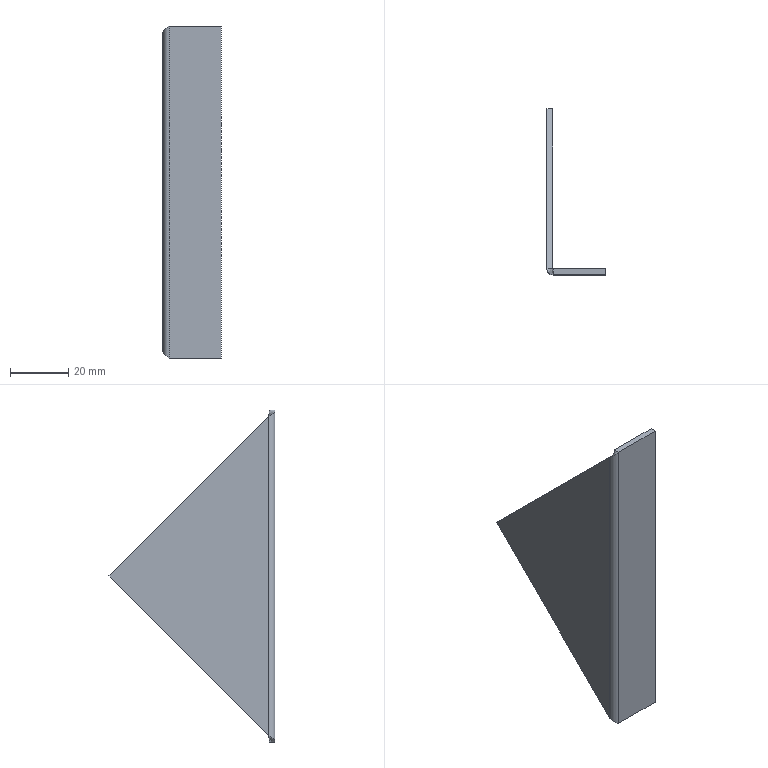Part | STEP file | Front Left Filler Piece | 1 solid | 13 faces | box 20 x 57.062 x 114.125 mm | volume 10515 mm3 | plane 9 | cylinder 2 | spline 2 | commonest cylinder face diameters 0.2 x1 4.2 x1
STEP:
#1=CARTESIAN_POINT('',(-2.,2.1,-54.962));
#2=VERTEX_POINT('',#1);
#3=CARTESIAN_POINT('',(-2.,2.1,54.962));
#4=VERTEX_POINT('',#3);
#5=CARTESIAN_POINT('',(-2.,2.1,0.));
#6=DIRECTION('',(0.,0.,1.));
#7=VECTOR('',#6,1000.);
#8=LINE('',#5,#7);
#9=EDGE_CURVE('',#2,#4,#8,.T.);
#10=ORIENTED_EDGE('',*,*,#9,.T.);
#11=CARTESIAN_POINT('',(-2.,57.062,0.));
#12=VERTEX_POINT('',#11);
#13=CARTESIAN_POINT('',(-2.,2.1,54.962));
#14=DIRECTION('',(0.,0.7071,-0.7071));
#15=VECTOR('',#14,1000.);
#16=LINE('',#13,#15);
#17=EDGE_CURVE('',#4,#12,#16,.T.);
#18=ORIENTED_EDGE('',*,*,#17,.T.);
#19=CARTESIAN_POINT('',(-2.,57.062,0.));
#20=DIRECTION('',(0.,-0.7071,-0.7071));
#21=VECTOR('',#20,1000.);
#22=LINE('',#19,#21);
#23=EDGE_CURVE('',#12,#2,#22,.T.);
#24=ORIENTED_EDGE('',*,*,#23,.T.);
#25=EDGE_LOOP('',(#10,#18,#24));
#26=FACE_OUTER_BOUND('',#25,.T.);
#27=CARTESIAN_POINT('',(-2.,0.,0.));
#28=DIRECTION('',(-1.,0.,0.));
#29=DIRECTION('',(0.,0.,1.));
#30=AXIS2_PLACEMENT_3D('',#27,#28,#29);
#31=PLANE('',#30);
#32=ADVANCED_FACE('',(#26),#31,.T.);
#33=CARTESIAN_POINT('',(0.,2.1,54.962));
#34=VERTEX_POINT('',#33);
#35=CARTESIAN_POINT('',(0.,57.062,0.));
#36=VERTEX_POINT('',#35);
#37=CARTESIAN_POINT('',(0.,57.062,0.));
#38=DIRECTION('',(0.,0.7071,-0.7071));
#39=VECTOR('',#38,1000.);
#40=LINE('',#37,#39);
#41=EDGE_CURVE('',#34,#36,#40,.T.);
#42=ORIENTED_EDGE('',*,*,#41,.T.);
#43=CARTESIAN_POINT('',(-2.,57.062,0.));
#44=DIRECTION('',(-1.,0.,0.));
#45=VECTOR('',#44,1000.);
#46=LINE('',#43,#45);
#47=EDGE_CURVE('',#36,#12,#46,.T.);
#48=ORIENTED_EDGE('',*,*,#47,.T.);
#49=ORIENTED_EDGE('',*,*,#17,.F.);
#50=CARTESIAN_POINT('',(-2.,2.1,54.962));
#51=DIRECTION('',(1.,0.,0.));
#52=VECTOR('',#51,1000.);
#53=LINE('',#50,#52);
#54=EDGE_CURVE('',#4,#34,#53,.T.);
#55=ORIENTED_EDGE('',*,*,#54,.T.);
#56=EDGE_LOOP('',(#42,#48,#49,#55));
#57=FACE_OUTER_BOUND('',#56,.T.);
#58=CARTESIAN_POINT('',(-2.,57.062,0.));
#59=DIRECTION('',(0.,0.7071,0.7071));
#60=DIRECTION('',(0.,-0.7071,0.7071));
#61=AXIS2_PLACEMENT_3D('',#58,#59,#60);
#62=PLANE('',#61);
#63=ADVANCED_FACE('',(#57),#62,.T.);
#64=CARTESIAN_POINT('',(0.1,0.,-57.062));
#65=VERTEX_POINT('',#64);
#66=CARTESIAN_POINT('',(0.1,0.,57.062));
#67=VERTEX_POINT('',#66);
#68=CARTESIAN_POINT('',(0.1,0.,-57.062));
#69=DIRECTION('',(0.,0.,1.));
#70=VECTOR('',#69,1000.);
#71=LINE('',#68,#70);
#72=EDGE_CURVE('',#65,#67,#71,.T.);
#73=ORIENTED_EDGE('',*,*,#72,.T.);
#74=CARTESIAN_POINT('',(0.1,0.,57.062));
#75=CARTESIAN_POINT('',(0.06419,0.,57.04));
#76=CARTESIAN_POINT('',(0.02837,0.0009165,57.017));
#77=CARTESIAN_POINT('',(-0.007394,0.002748,56.994));
#78=CARTESIAN_POINT('',(-0.04316,0.004579,56.971));
#79=CARTESIAN_POINT('',(-0.07888,0.007326,56.948));
#80=CARTESIAN_POINT('',(-0.1145,0.01098,56.926));
#81=CARTESIAN_POINT('',(-0.1501,0.01464,56.903));
#82=CARTESIAN_POINT('',(-0.1857,0.01921,56.88));
#83=CARTESIAN_POINT('',(-0.2211,0.02469,56.857));
#84=CARTESIAN_POINT('',(-0.2565,0.03016,56.834));
#85=CARTESIAN_POINT('',(-0.2917,0.03655,56.812));
#86=CARTESIAN_POINT('',(-0.3268,0.04382,56.789));
#87=CARTESIAN_POINT('',(-0.3618,0.0511,56.766));
#88=CARTESIAN_POINT('',(-0.3967,0.05928,56.743));
#89=CARTESIAN_POINT('',(-0.4314,0.06834,56.72));
#90=CARTESIAN_POINT('',(-0.466,0.0774,56.698));
#91=CARTESIAN_POINT('',(-0.5004,0.08735,56.675));
#92=CARTESIAN_POINT('',(-0.5346,0.09817,56.652));
#93=CARTESIAN_POINT('',(-0.5687,0.109,56.629));
#94=CARTESIAN_POINT('',(-0.6026,0.1207,56.606));
#95=CARTESIAN_POINT('',(-0.6361,0.1332,56.584));
#96=CARTESIAN_POINT('',(-0.6697,0.1458,56.561));
#97=CARTESIAN_POINT('',(-0.7029,0.1592,56.538));
#98=CARTESIAN_POINT('',(-0.7357,0.1735,56.515));
#99=CARTESIAN_POINT('',(-0.7686,0.1877,56.492));
#100=CARTESIAN_POINT('',(-0.8011,0.2028,56.47));
#101=CARTESIAN_POINT('',(-0.8332,0.2187,56.447));
#102=CARTESIAN_POINT('',(-0.8652,0.2346,56.424));
#103=CARTESIAN_POINT('',(-0.8969,0.2514,56.401));
#104=CARTESIAN_POINT('',(-0.9282,0.2689,56.378));
#105=CARTESIAN_POINT('',(-0.9594,0.2864,56.356));
#106=CARTESIAN_POINT('',(-0.9902,0.3048,56.333));
#107=CARTESIAN_POINT('',(-1.02,0.3239,56.31));
#108=CARTESIAN_POINT('',(-1.051,0.343,56.287));
#109=CARTESIAN_POINT('',(-1.081,0.3629,56.264));
#110=CARTESIAN_POINT('',(-1.11,0.3835,56.242));
#111=CARTESIAN_POINT('',(-1.139,0.4041,56.219));
#112=CARTESIAN_POINT('',(-1.168,0.4255,56.196));
#113=CARTESIAN_POINT('',(-1.196,0.4476,56.173));
#114=CARTESIAN_POINT('',(-1.224,0.4697,56.15));
#115=CARTESIAN_POINT('',(-1.252,0.4926,56.128));
#116=CARTESIAN_POINT('',(-1.279,0.5161,56.105));
#117=CARTESIAN_POINT('',(-1.306,0.5396,56.082));
#118=CARTESIAN_POINT('',(-1.332,0.5638,56.059));
#119=CARTESIAN_POINT('',(-1.358,0.5887,56.036));
#120=CARTESIAN_POINT('',(-1.384,0.6135,56.014));
#121=CARTESIAN_POINT('',(-1.409,0.639,55.991));
#122=CARTESIAN_POINT('',(-1.433,0.6652,55.968));
#123=CARTESIAN_POINT('',(-1.458,0.6913,55.945));
#124=CARTESIAN_POINT('',(-1.482,0.7181,55.922));
#125=CARTESIAN_POINT('',(-1.505,0.7455,55.9));
#126=CARTESIAN_POINT('',(-1.528,0.7729,55.877));
#127=CARTESIAN_POINT('',(-1.55,0.8008,55.854));
#128=CARTESIAN_POINT('',(-1.572,0.8293,55.831));
#129=CARTESIAN_POINT('',(-1.594,0.8578,55.808));
#130=CARTESIAN_POINT('',(-1.615,0.8869,55.786));
#131=CARTESIAN_POINT('',(-1.635,0.9165,55.763));
#132=CARTESIAN_POINT('',(-1.655,0.9461,55.74));
#133=CARTESIAN_POINT('',(-1.674,0.9762,55.717));
#134=CARTESIAN_POINT('',(-1.693,1.007,55.694));
#135=CARTESIAN_POINT('',(-1.712,1.037,55.672));
#136=CARTESIAN_POINT('',(-1.73,1.068,55.649));
#137=CARTESIAN_POINT('',(-1.747,1.1,55.626));
#138=CARTESIAN_POINT('',(-1.764,1.131,55.603));
#139=CARTESIAN_POINT('',(-1.78,1.163,55.58));
#140=CARTESIAN_POINT('',(-1.795,1.196,55.558));
#141=CARTESIAN_POINT('',(-1.811,1.228,55.535));
#142=CARTESIAN_POINT('',(-1.825,1.261,55.512));
#143=CARTESIAN_POINT('',(-1.839,1.294,55.489));
#144=CARTESIAN_POINT('',(-1.846,1.31,55.478));
#145=CARTESIAN_POINT('',(-1.853,1.327,55.466));
#146=CARTESIAN_POINT('',(-1.859,1.344,55.455));
#147=CARTESIAN_POINT('',(-1.872,1.377,55.432));
#148=CARTESIAN_POINT('',(-1.884,1.411,55.409));
#149=CARTESIAN_POINT('',(-1.895,1.445,55.387));
#150=CARTESIAN_POINT('',(-1.906,1.479,55.364));
#151=CARTESIAN_POINT('',(-1.917,1.513,55.341));
#152=CARTESIAN_POINT('',(-1.926,1.548,55.318));
#153=CARTESIAN_POINT('',(-1.935,1.582,55.295));
#154=CARTESIAN_POINT('',(-1.944,1.617,55.273));
#155=CARTESIAN_POINT('',(-1.952,1.652,55.25));
#156=CARTESIAN_POINT('',(-1.959,1.687,55.227));
#157=CARTESIAN_POINT('',(-1.966,1.722,55.204));
#158=CARTESIAN_POINT('',(-1.972,1.758,55.181));
#159=CARTESIAN_POINT('',(-1.978,1.793,55.159));
#160=CARTESIAN_POINT('',(-1.983,1.828,55.136));
#161=CARTESIAN_POINT('',(-1.987,1.864,55.113));
#162=CARTESIAN_POINT('',(-1.991,1.903,55.088));
#163=CARTESIAN_POINT('',(-1.994,1.942,55.063));
#164=CARTESIAN_POINT('',(-1.997,1.982,55.038));
#165=CARTESIAN_POINT('',(-1.999,2.021,55.013));
#166=CARTESIAN_POINT('',(-2.,2.061,54.988));
#167=CARTESIAN_POINT('',(-2.,2.1,54.962));
#168=B_SPLINE_CURVE_WITH_KNOTS('',3,(#74,#75,#76,#77,#78,#79,#80,#81,#82,#83,#84,#85,#86,#87,#88,#89,#90,#91,#92,#93,#94,#95,#96,#97,#98,#99,#100,#101,#102,#103,#104,#105,#106,#107,#108,#109,#110,#111,#112,#113,#114,#115,#116,#117,#118,#119,#120,#121,#122,#123,#124,#125,#126,#127,#128,#129,#130,#131,#132,#133,#134,#135,#136,#137,#138,#139,#140,#141,#142,#143,#144,#145,#146,#147,#148,#149,#150,#151,#152,#153,#154,#155,#156,#157,#158,#159,#160,#161,#162,#163,#164,#165,#166,#167),.UNSPECIFIED.,.F.,.F.,(4,3,3,3,3,3,3,3,3,3,3,3,3,3,3,3,3,3,3,3,3,3,3,3,3,3,3,3,3,3,3,4),(0.,0.0001274,0.0002547,0.0003821,0.0005094,0.0006368,0.0007641,0.0008915,0.001019,0.001146,0.001274,0.001401,0.001528,0.001656,0.001783,0.00191,0.002038,0.002165,0.002292,0.00242,0.002547,0.002674,0.002802,0.002929,0.002993,0.00312,0.003248,0.003375,0.003502,0.00363,0.00377,0.00391),.UNSPECIFIED.);
#169=EDGE_CURVE('',#67,#4,#168,.T.);
#170=ORIENTED_EDGE('',*,*,#169,.T.);
#171=ORIENTED_EDGE('',*,*,#9,.F.);
#172=CARTESIAN_POINT('',(-2.,2.1,-54.962));
#173=CARTESIAN_POINT('',(-2.,2.064,-54.985));
#174=CARTESIAN_POINT('',(-1.999,2.028,-55.008));
#175=CARTESIAN_POINT('',(-1.997,1.993,-55.031));
#176=CARTESIAN_POINT('',(-1.995,1.957,-55.054));
#177=CARTESIAN_POINT('',(-1.993,1.921,-55.076));
#178=CARTESIAN_POINT('',(-1.989,1.885,-55.099));
#179=CARTESIAN_POINT('',(-1.985,1.85,-55.122));
#180=CARTESIAN_POINT('',(-1.981,1.814,-55.145));
#181=CARTESIAN_POINT('',(-1.975,1.779,-55.168));
#182=CARTESIAN_POINT('',(-1.97,1.744,-55.19));
#183=CARTESIAN_POINT('',(-1.963,1.708,-55.213));
#184=CARTESIAN_POINT('',(-1.956,1.673,-55.236));
#185=CARTESIAN_POINT('',(-1.949,1.638,-55.259));
#186=CARTESIAN_POINT('',(-1.941,1.603,-55.282));
#187=CARTESIAN_POINT('',(-1.932,1.569,-55.304));
#188=CARTESIAN_POINT('',(-1.923,1.534,-55.327));
#189=CARTESIAN_POINT('',(-1.913,1.5,-55.35));
#190=CARTESIAN_POINT('',(-1.902,1.465,-55.373));
#191=CARTESIAN_POINT('',(-1.891,1.431,-55.396));
#192=CARTESIAN_POINT('',(-1.879,1.397,-55.418));
#193=CARTESIAN_POINT('',(-1.867,1.364,-55.441));
#194=CARTESIAN_POINT('',(-1.854,1.33,-55.464));
#195=CARTESIAN_POINT('',(-1.841,1.297,-55.487));
#196=CARTESIAN_POINT('',(-1.827,1.264,-55.51));
#197=CARTESIAN_POINT('',(-1.812,1.231,-55.532));
#198=CARTESIAN_POINT('',(-1.797,1.199,-55.555));
#199=CARTESIAN_POINT('',(-1.781,1.167,-55.578));
#200=CARTESIAN_POINT('',(-1.765,1.135,-55.601));
#201=CARTESIAN_POINT('',(-1.749,1.103,-55.624));
#202=CARTESIAN_POINT('',(-1.731,1.072,-55.646));
#203=CARTESIAN_POINT('',(-1.714,1.041,-55.669));
#204=CARTESIAN_POINT('',(-1.695,1.01,-55.692));
#205=CARTESIAN_POINT('',(-1.676,0.9795,-55.715));
#206=CARTESIAN_POINT('',(-1.657,0.9493,-55.738));
#207=CARTESIAN_POINT('',(-1.637,0.9195,-55.76));
#208=CARTESIAN_POINT('',(-1.616,0.8902,-55.783));
#209=CARTESIAN_POINT('',(-1.596,0.8609,-55.806));
#210=CARTESIAN_POINT('',(-1.574,0.8322,-55.829));
#211=CARTESIAN_POINT('',(-1.552,0.804,-55.852));
#212=CARTESIAN_POINT('',(-1.53,0.7758,-55.874));
#213=CARTESIAN_POINT('',(-1.507,0.7482,-55.897));
#214=CARTESIAN_POINT('',(-1.484,0.7212,-55.92));
#215=CARTESIAN_POINT('',(-1.46,0.6942,-55.943));
#216=CARTESIAN_POINT('',(-1.436,0.6677,-55.966));
#217=CARTESIAN_POINT('',(-1.411,0.642,-55.988));
#218=CARTESIAN_POINT('',(-1.386,0.6162,-56.011));
#219=CARTESIAN_POINT('',(-1.361,0.5911,-56.034));
#220=CARTESIAN_POINT('',(-1.335,0.5666,-56.057));
#221=CARTESIAN_POINT('',(-1.309,0.5421,-56.08));
#222=CARTESIAN_POINT('',(-1.282,0.5183,-56.102));
#223=CARTESIAN_POINT('',(-1.255,0.4952,-56.125));
#224=CARTESIAN_POINT('',(-1.227,0.4721,-56.148));
#225=CARTESIAN_POINT('',(-1.199,0.4497,-56.171));
#226=CARTESIAN_POINT('',(-1.171,0.4281,-56.194));
#227=CARTESIAN_POINT('',(-1.142,0.4064,-56.216));
#228=CARTESIAN_POINT('',(-1.113,0.3854,-56.239));
#229=CARTESIAN_POINT('',(-1.083,0.3653,-56.262));
#230=CARTESIAN_POINT('',(-1.054,0.3451,-56.285));
#231=CARTESIAN_POINT('',(-1.024,0.3256,-56.308));
#232=CARTESIAN_POINT('',(-0.9932,0.307,-56.33));
#233=CARTESIAN_POINT('',(-0.9627,0.2884,-56.353));
#234=CARTESIAN_POINT('',(-0.9316,0.2705,-56.376));
#235=CARTESIAN_POINT('',(-0.9001,0.2534,-56.399));
#236=CARTESIAN_POINT('',(-0.8686,0.2364,-56.422));
#237=CARTESIAN_POINT('',(-0.8367,0.2201,-56.444));
#238=CARTESIAN_POINT('',(-0.8044,0.2047,-56.467));
#239=CARTESIAN_POINT('',(-0.772,0.1893,-56.49));
#240=CARTESIAN_POINT('',(-0.7393,0.1747,-56.513));
#241=CARTESIAN_POINT('',(-0.7063,0.1609,-56.536));
#242=CARTESIAN_POINT('',(-0.6897,0.1541,-56.547));
#243=CARTESIAN_POINT('',(-0.6731,0.1474,-56.558));
#244=CARTESIAN_POINT('',(-0.6564,0.141,-56.57));
#245=CARTESIAN_POINT('',(-0.623,0.1281,-56.593));
#246=CARTESIAN_POINT('',(-0.5893,0.116,-56.615));
#247=CARTESIAN_POINT('',(-0.5552,0.1048,-56.638));
#248=CARTESIAN_POINT('',(-0.5212,0.09366,-56.661));
#249=CARTESIAN_POINT('',(-0.4869,0.08336,-56.684));
#250=CARTESIAN_POINT('',(-0.4523,0.07394,-56.707));
#251=CARTESIAN_POINT('',(-0.4178,0.06452,-56.729));
#252=CARTESIAN_POINT('',(-0.383,0.05598,-56.752));
#253=CARTESIAN_POINT('',(-0.348,0.04834,-56.775));
#254=CARTESIAN_POINT('',(-0.313,0.0407,-56.798));
#255=CARTESIAN_POINT('',(-0.2778,0.03396,-56.821));
#256=CARTESIAN_POINT('',(-0.2425,0.02812,-56.843));
#257=CARTESIAN_POINT('',(-0.2072,0.02228,-56.866));
#258=CARTESIAN_POINT('',(-0.1717,0.01734,-56.889));
#259=CARTESIAN_POINT('',(-0.1361,0.01331,-56.912));
#260=CARTESIAN_POINT('',(-0.09695,0.008885,-56.937));
#261=CARTESIAN_POINT('',(-0.05768,0.005558,-56.962));
#262=CARTESIAN_POINT('',(-0.01836,0.003338,-56.987));
#263=CARTESIAN_POINT('',(0.02105,0.001114,-57.012));
#264=CARTESIAN_POINT('',(0.06053,0.,-57.037));
#265=CARTESIAN_POINT('',(0.1,0.,-57.062));
#266=B_SPLINE_CURVE_WITH_KNOTS('',3,(#172,#173,#174,#175,#176,#177,#178,#179,#180,#181,#182,#183,#184,#185,#186,#187,#188,#189,#190,#191,#192,#193,#194,#195,#196,#197,#198,#199,#200,#201,#202,#203,#204,#205,#206,#207,#208,#209,#210,#211,#212,#213,#214,#215,#216,#217,#218,#219,#220,#221,#222,#223,#224,#225,#226,#227,#228,#229,#230,#231,#232,#233,#234,#235,#236,#237,#238,#239,#240,#241,#242,#243,#244,#245,#246,#247,#248,#249,#250,#251,#252,#253,#254,#255,#256,#257,#258,#259,#260,#261,#262,#263,#264,#265),.UNSPECIFIED.,.F.,.F.,(4,3,3,3,3,3,3,3,3,3,3,3,3,3,3,3,3,3,3,3,3,3,3,3,3,3,3,3,3,3,3,4),(0.,0.0001274,0.0002547,0.0003821,0.0005094,0.0006368,0.0007641,0.0008915,0.001019,0.001146,0.001274,0.001401,0.001528,0.001656,0.001783,0.00191,0.002038,0.002165,0.002292,0.00242,0.002547,0.002674,0.002802,0.002929,0.002993,0.00312,0.003248,0.003375,0.003502,0.00363,0.00377,0.00391),.UNSPECIFIED.);
#267=EDGE_CURVE('',#2,#65,#266,.T.);
#268=ORIENTED_EDGE('',*,*,#267,.T.);
#269=EDGE_LOOP('',(#73,#170,#171,#268));
#270=FACE_OUTER_BOUND('',#269,.T.);
#271=CARTESIAN_POINT('',(0.1,2.1,-57.062));
#272=DIRECTION('',(0.,0.,-1.));
#273=DIRECTION('',(-1.,0.,0.));
#274=AXIS2_PLACEMENT_3D('',#271,#272,#273);
#275=CYLINDRICAL_SURFACE('',#274,2.1);
#276=ADVANCED_FACE('',(#270),#275,.T.);
#277=ORIENTED_EDGE('',*,*,#23,.F.);
#278=ORIENTED_EDGE('',*,*,#47,.F.);
#279=CARTESIAN_POINT('',(0.,2.1,-54.962));
#280=VERTEX_POINT('',#279);
#281=CARTESIAN_POINT('',(0.,0.,-57.062));
#282=DIRECTION('',(0.,-0.7071,-0.7071));
#283=VECTOR('',#282,1000.);
#284=LINE('',#281,#283);
#285=EDGE_CURVE('',#36,#280,#284,.T.);
#286=ORIENTED_EDGE('',*,*,#285,.T.);
#287=CARTESIAN_POINT('',(-2.,2.1,-54.962));
#288=DIRECTION('',(-1.,0.,0.));
#289=VECTOR('',#288,1000.);
#290=LINE('',#287,#289);
#291=EDGE_CURVE('',#280,#2,#290,.T.);
#292=ORIENTED_EDGE('',*,*,#291,.T.);
#293=EDGE_LOOP('',(#277,#278,#286,#292));
#294=FACE_OUTER_BOUND('',#293,.T.);
#295=CARTESIAN_POINT('',(-2.,0.,-57.062));
#296=DIRECTION('',(0.,0.7071,-0.7071));
#297=DIRECTION('',(0.,0.7071,0.7071));
#298=AXIS2_PLACEMENT_3D('',#295,#296,#297);
#299=PLANE('',#298);
#300=ADVANCED_FACE('',(#294),#299,.T.);
#301=ORIENTED_EDGE('',*,*,#285,.F.);
#302=ORIENTED_EDGE('',*,*,#41,.F.);
#303=CARTESIAN_POINT('',(0.,2.1,0.));
#304=DIRECTION('',(0.,0.,1.));
#305=VECTOR('',#304,1000.);
#306=LINE('',#303,#305);
#307=EDGE_CURVE('',#280,#34,#306,.T.);
#308=ORIENTED_EDGE('',*,*,#307,.F.);
#309=EDGE_LOOP('',(#301,#302,#308));
#310=FACE_OUTER_BOUND('',#309,.T.);
#311=CARTESIAN_POINT('',(0.,0.,0.));
#312=DIRECTION('',(-1.,0.,0.));
#313=DIRECTION('',(0.,0.,1.));
#314=AXIS2_PLACEMENT_3D('',#311,#312,#313);
#315=PLANE('',#314);
#316=ADVANCED_FACE('',(#310),#315,.F.);
#317=CARTESIAN_POINT('',(0.1,2.,57.062));
#318=VERTEX_POINT('',#317);
#319=CARTESIAN_POINT('',(0.,2.1,54.962));
#320=CARTESIAN_POINT('',(0.,2.074,55.312));
#321=CARTESIAN_POINT('',(0.01078,2.048,55.662));
#322=CARTESIAN_POINT('',(0.0478,2.011,56.362));
#323=CARTESIAN_POINT('',(0.07382,2.,56.712));
#324=CARTESIAN_POINT('',(0.1,2.,57.062));
#325=B_SPLINE_CURVE_WITH_KNOTS('',3,(#319,#320,#321,#322,#323,#324),.UNSPECIFIED.,.F.,.F.,(4,2,4),(0.,0.5,1.),.UNSPECIFIED.);
#326=EDGE_CURVE('',#34,#318,#325,.T.);
#327=ORIENTED_EDGE('',*,*,#326,.F.);
#328=ORIENTED_EDGE('',*,*,#54,.F.);
#329=ORIENTED_EDGE('',*,*,#169,.F.);
#330=CARTESIAN_POINT('',(0.1,0.99,57.062));
#331=DIRECTION('',(0.,-1.,0.));
#332=VECTOR('',#331,1000.);
#333=LINE('',#330,#332);
#334=EDGE_CURVE('',#318,#67,#333,.T.);
#335=ORIENTED_EDGE('',*,*,#334,.F.);
#336=EDGE_LOOP('',(#327,#328,#329,#335));
#337=FACE_OUTER_BOUND('',#336,.T.);
#338=CARTESIAN_POINT('',(-2.02,2.1,54.962));
#339=CARTESIAN_POINT('',(-2.02,1.822,55.137));
#340=CARTESIAN_POINT('',(-1.965,1.545,55.312));
#341=CARTESIAN_POINT('',(-1.752,1.032,55.662));
#342=CARTESIAN_POINT('',(-1.595,0.7972,55.837));
#343=CARTESIAN_POINT('',(-1.203,0.4047,56.187));
#344=CARTESIAN_POINT('',(-0.9677,0.2476,56.362));
#345=CARTESIAN_POINT('',(-0.4549,0.03518,56.712));
#346=CARTESIAN_POINT('',(-0.1775,-0.02,56.887));
#347=CARTESIAN_POINT('',(0.1,-0.02,57.062));
#348=CARTESIAN_POINT('',(-2.,2.1,54.962));
#349=CARTESIAN_POINT('',(-2.,1.825,55.137));
#350=CARTESIAN_POINT('',(-1.945,1.55,55.312));
#351=CARTESIAN_POINT('',(-1.735,1.042,55.662));
#352=CARTESIAN_POINT('',(-1.579,0.8095,55.837));
#353=CARTESIAN_POINT('',(-1.191,0.4207,56.187));
#354=CARTESIAN_POINT('',(-0.9576,0.265,56.362));
#355=CARTESIAN_POINT('',(-0.4497,0.05466,56.712));
#356=CARTESIAN_POINT('',(-0.1749,0.,56.887));
#357=CARTESIAN_POINT('',(0.1,0.,57.062));
#358=CARTESIAN_POINT('',(0.,2.1,54.962));
#359=CARTESIAN_POINT('',(0.,2.087,55.137));
#360=CARTESIAN_POINT('',(0.002603,2.074,55.312));
#361=CARTESIAN_POINT('',(0.01262,2.05,55.662));
#362=CARTESIAN_POINT('',(0.02003,2.039,55.837));
#363=CARTESIAN_POINT('',(0.03855,2.02,56.187));
#364=CARTESIAN_POINT('',(0.04964,2.013,56.362));
#365=CARTESIAN_POINT('',(0.07383,2.003,56.712));
#366=CARTESIAN_POINT('',(0.08691,2.,56.887));
#367=CARTESIAN_POINT('',(0.1,2.,57.062));
#368=B_SPLINE_SURFACE_WITH_KNOTS('',1,3,((#338,#339,#340,#341,#342,#343,#344,#345,#346,#347),(#348,#349,#350,#351,#352,#353,#354,#355,#356,#357),(#358,#359,#360,#361,#362,#363,#364,#365,#366,#367)),.UNSPECIFIED.,.F.,.F.,.F.,(2,1,2),(4,2,2,2,4),(-0.01,0.,1.),(0.,0.25,0.5,0.75,1.),.UNSPECIFIED.);
#369=ADVANCED_FACE('',(#337),#368,.F.);
#370=CARTESIAN_POINT('',(18.,0.,-57.062));
#371=VERTEX_POINT('',#370);
#372=CARTESIAN_POINT('',(0.,0.,-57.062));
#373=DIRECTION('',(-1.,0.,0.));
#374=VECTOR('',#373,1000.);
#375=LINE('',#372,#374);
#376=EDGE_CURVE('',#371,#65,#375,.T.);
#377=ORIENTED_EDGE('',*,*,#376,.F.);
#378=CARTESIAN_POINT('',(18.,0.,57.062));
#379=VERTEX_POINT('',#378);
#380=CARTESIAN_POINT('',(18.,0.,0.));
#381=DIRECTION('',(0.,0.,-1.));
#382=VECTOR('',#381,1000.);
#383=LINE('',#380,#382);
#384=EDGE_CURVE('',#379,#371,#383,.T.);
#385=ORIENTED_EDGE('',*,*,#384,.F.);
#386=CARTESIAN_POINT('',(0.,0.,57.062));
#387=DIRECTION('',(1.,0.,0.));
#388=VECTOR('',#387,1000.);
#389=LINE('',#386,#388);
#390=EDGE_CURVE('',#67,#379,#389,.T.);
#391=ORIENTED_EDGE('',*,*,#390,.F.);
#392=ORIENTED_EDGE('',*,*,#72,.F.);
#393=EDGE_LOOP('',(#377,#385,#391,#392));
#394=FACE_OUTER_BOUND('',#393,.T.);
#395=CARTESIAN_POINT('',(0.,0.,0.));
#396=DIRECTION('',(0.,1.,0.));
#397=DIRECTION('',(-1.,0.,0.));
#398=AXIS2_PLACEMENT_3D('',#395,#396,#397);
#399=PLANE('',#398);
#400=ADVANCED_FACE('',(#394),#399,.F.);
#401=CARTESIAN_POINT('',(0.1,2.,-57.062));
#402=VERTEX_POINT('',#401);
#403=CARTESIAN_POINT('',(0.1,0.99,-57.062));
#404=DIRECTION('',(0.,1.,0.));
#405=VECTOR('',#404,1000.);
#406=LINE('',#403,#405);
#407=EDGE_CURVE('',#65,#402,#406,.T.);
#408=ORIENTED_EDGE('',*,*,#407,.F.);
#409=ORIENTED_EDGE('',*,*,#267,.F.);
#410=ORIENTED_EDGE('',*,*,#291,.F.);
#411=CARTESIAN_POINT('',(0.1,2.,-57.062));
#412=CARTESIAN_POINT('',(0.07382,2.,-56.712));
#413=CARTESIAN_POINT('',(0.0478,2.011,-56.362));
#414=CARTESIAN_POINT('',(0.01078,2.048,-55.662));
#415=CARTESIAN_POINT('',(0.,2.074,-55.312));
#416=CARTESIAN_POINT('',(0.,2.1,-54.962));
#417=B_SPLINE_CURVE_WITH_KNOTS('',3,(#411,#412,#413,#414,#415,#416),.UNSPECIFIED.,.F.,.F.,(4,2,4),(0.,0.5,1.),.UNSPECIFIED.);
#418=EDGE_CURVE('',#402,#280,#417,.T.);
#419=ORIENTED_EDGE('',*,*,#418,.F.);
#420=EDGE_LOOP('',(#408,#409,#410,#419));
#421=FACE_OUTER_BOUND('',#420,.T.);
#422=CARTESIAN_POINT('',(0.1,-0.02,-57.062));
#423=CARTESIAN_POINT('',(-0.1775,-0.02,-56.887));
#424=CARTESIAN_POINT('',(-0.4549,0.03518,-56.712));
#425=CARTESIAN_POINT('',(-0.9677,0.2476,-56.362));
#426=CARTESIAN_POINT('',(-1.203,0.4047,-56.187));
#427=CARTESIAN_POINT('',(-1.595,0.7972,-55.837));
#428=CARTESIAN_POINT('',(-1.752,1.032,-55.662));
#429=CARTESIAN_POINT('',(-1.965,1.545,-55.312));
#430=CARTESIAN_POINT('',(-2.02,1.822,-55.137));
#431=CARTESIAN_POINT('',(-2.02,2.1,-54.962));
#432=CARTESIAN_POINT('',(0.1,0.,-57.062));
#433=CARTESIAN_POINT('',(-0.1749,0.,-56.887));
#434=CARTESIAN_POINT('',(-0.4497,0.05466,-56.712));
#435=CARTESIAN_POINT('',(-0.9576,0.265,-56.362));
#436=CARTESIAN_POINT('',(-1.191,0.4207,-56.187));
#437=CARTESIAN_POINT('',(-1.579,0.8095,-55.837));
#438=CARTESIAN_POINT('',(-1.735,1.042,-55.662));
#439=CARTESIAN_POINT('',(-1.945,1.55,-55.312));
#440=CARTESIAN_POINT('',(-2.,1.825,-55.137));
#441=CARTESIAN_POINT('',(-2.,2.1,-54.962));
#442=CARTESIAN_POINT('',(0.1,2.,-57.062));
#443=CARTESIAN_POINT('',(0.08691,2.,-56.887));
#444=CARTESIAN_POINT('',(0.07383,2.003,-56.712));
#445=CARTESIAN_POINT('',(0.04964,2.013,-56.362));
#446=CARTESIAN_POINT('',(0.03855,2.02,-56.187));
#447=CARTESIAN_POINT('',(0.02003,2.039,-55.837));
#448=CARTESIAN_POINT('',(0.01262,2.05,-55.662));
#449=CARTESIAN_POINT('',(0.002603,2.074,-55.312));
#450=CARTESIAN_POINT('',(0.,2.087,-55.137));
#451=CARTESIAN_POINT('',(0.,2.1,-54.962));
#452=B_SPLINE_SURFACE_WITH_KNOTS('',1,3,((#422,#423,#424,#425,#426,#427,#428,#429,#430,#431),(#432,#433,#434,#435,#436,#437,#438,#439,#440,#441),(#442,#443,#444,#445,#446,#447,#448,#449,#450,#451)),.UNSPECIFIED.,.F.,.F.,.F.,(2,1,2),(4,2,2,2,4),(-0.01,0.,1.),(0.,0.25,0.5,0.75,1.),.UNSPECIFIED.);
#453=ADVANCED_FACE('',(#421),#452,.F.);
#454=ORIENTED_EDGE('',*,*,#326,.T.);
#455=CARTESIAN_POINT('',(0.1,2.,-57.062));
#456=DIRECTION('',(0.,0.,1.));
#457=VECTOR('',#456,1000.);
#458=LINE('',#455,#457);
#459=EDGE_CURVE('',#402,#318,#458,.T.);
#460=ORIENTED_EDGE('',*,*,#459,.F.);
#461=ORIENTED_EDGE('',*,*,#418,.T.);
#462=ORIENTED_EDGE('',*,*,#307,.T.);
#463=EDGE_LOOP('',(#454,#460,#461,#462));
#464=FACE_OUTER_BOUND('',#463,.T.);
#465=CARTESIAN_POINT('',(0.1,2.1,-57.062));
#466=DIRECTION('',(0.,0.,-1.));
#467=DIRECTION('',(-1.,0.,0.));
#468=AXIS2_PLACEMENT_3D('',#465,#466,#467);
#469=CYLINDRICAL_SURFACE('',#468,0.1);
#470=ADVANCED_FACE('',(#464),#469,.F.);
#471=ORIENTED_EDGE('',*,*,#390,.T.);
#472=CARTESIAN_POINT('',(18.,2.,57.062));
#473=VERTEX_POINT('',#472);
#474=CARTESIAN_POINT('',(18.,0.,57.062));
#475=DIRECTION('',(0.,-1.,0.));
#476=VECTOR('',#475,1000.);
#477=LINE('',#474,#476);
#478=EDGE_CURVE('',#473,#379,#477,.T.);
#479=ORIENTED_EDGE('',*,*,#478,.F.);
#480=CARTESIAN_POINT('',(0.,2.,57.062));
#481=DIRECTION('',(1.,0.,0.));
#482=VECTOR('',#481,1000.);
#483=LINE('',#480,#482);
#484=EDGE_CURVE('',#318,#473,#483,.T.);
#485=ORIENTED_EDGE('',*,*,#484,.F.);
#486=ORIENTED_EDGE('',*,*,#334,.T.);
#487=EDGE_LOOP('',(#471,#479,#485,#486));
#488=FACE_OUTER_BOUND('',#487,.T.);
#489=CARTESIAN_POINT('',(0.,0.,57.062));
#490=DIRECTION('',(0.,0.,-1.));
#491=DIRECTION('',(-1.,0.,0.));
#492=AXIS2_PLACEMENT_3D('',#489,#490,#491);
#493=PLANE('',#492);
#494=ADVANCED_FACE('',(#488),#493,.F.);
#495=CARTESIAN_POINT('',(18.,2.,-57.062));
#496=VERTEX_POINT('',#495);
#497=CARTESIAN_POINT('',(18.,2.,-57.062));
#498=DIRECTION('',(-1.,0.,0.));
#499=VECTOR('',#498,1000.);
#500=LINE('',#497,#499);
#501=EDGE_CURVE('',#496,#402,#500,.T.);
#502=ORIENTED_EDGE('',*,*,#501,.F.);
#503=CARTESIAN_POINT('',(18.,0.,-57.062));
#504=DIRECTION('',(0.,1.,0.));
#505=VECTOR('',#504,1000.);
#506=LINE('',#503,#505);
#507=EDGE_CURVE('',#371,#496,#506,.T.);
#508=ORIENTED_EDGE('',*,*,#507,.F.);
#509=ORIENTED_EDGE('',*,*,#376,.T.);
#510=ORIENTED_EDGE('',*,*,#407,.T.);
#511=EDGE_LOOP('',(#502,#508,#509,#510));
#512=FACE_OUTER_BOUND('',#511,.T.);
#513=CARTESIAN_POINT('',(18.,0.,-57.062));
#514=DIRECTION('',(0.,0.,1.));
#515=DIRECTION('',(1.,0.,0.));
#516=AXIS2_PLACEMENT_3D('',#513,#514,#515);
#517=PLANE('',#516);
#518=ADVANCED_FACE('',(#512),#517,.F.);
#519=ORIENTED_EDGE('',*,*,#478,.T.);
#520=ORIENTED_EDGE('',*,*,#384,.T.);
#521=ORIENTED_EDGE('',*,*,#507,.T.);
#522=CARTESIAN_POINT('',(18.,2.,57.062));
#523=DIRECTION('',(0.,0.,-1.));
#524=VECTOR('',#523,1000.);
#525=LINE('',#522,#524);
#526=EDGE_CURVE('',#473,#496,#525,.T.);
#527=ORIENTED_EDGE('',*,*,#526,.F.);
#528=EDGE_LOOP('',(#519,#520,#521,#527));
#529=FACE_OUTER_BOUND('',#528,.T.);
#530=CARTESIAN_POINT('',(18.,0.,57.062));
#531=DIRECTION('',(-1.,0.,0.));
#532=DIRECTION('',(0.,-1.,0.));
#533=AXIS2_PLACEMENT_3D('',#530,#531,#532);
#534=PLANE('',#533);
#535=ADVANCED_FACE('',(#529),#534,.F.);
#536=ORIENTED_EDGE('',*,*,#484,.T.);
#537=ORIENTED_EDGE('',*,*,#526,.T.);
#538=ORIENTED_EDGE('',*,*,#501,.T.);
#539=ORIENTED_EDGE('',*,*,#459,.T.);
#540=EDGE_LOOP('',(#536,#537,#538,#539));
#541=FACE_OUTER_BOUND('',#540,.T.);
#542=CARTESIAN_POINT('',(0.,2.,0.));
#543=DIRECTION('',(0.,1.,0.));
#544=DIRECTION('',(-1.,0.,0.));
#545=AXIS2_PLACEMENT_3D('',#542,#543,#544);
#546=PLANE('',#545);
#547=ADVANCED_FACE('',(#541),#546,.T.);
#548=CLOSED_SHELL('',(#32,#63,#276,#300,#316,#369,#400,#453,#470,#494,#518,#535,#547));
#549=MANIFOLD_SOLID_BREP('',#548);
#550=CARTESIAN_POINT('',(0.,0.,0.));
#551=DIRECTION('',(0.,0.,1.));
#552=DIRECTION('',(1.,0.,0.));
#553=AXIS2_PLACEMENT_3D('',#550,#551,#552);
#554=(LENGTH_UNIT()NAMED_UNIT(*)SI_UNIT(.MILLI.,.METRE.));
#555=UNCERTAINTY_MEASURE_WITH_UNIT(LENGTH_MEASURE(0.00001),#554,'','');
#556=(NAMED_UNIT(*)PLANE_ANGLE_UNIT()SI_UNIT($,.RADIAN.));
#557=(NAMED_UNIT(*)SI_UNIT($,.STERADIAN.)SOLID_ANGLE_UNIT());
#558=(GEOMETRIC_REPRESENTATION_CONTEXT(3)GLOBAL_UNCERTAINTY_ASSIGNED_CONTEXT((#555))GLOBAL_UNIT_ASSIGNED_CONTEXT((#554,#556,#557))REPRESENTATION_CONTEXT('',''));
#559=ADVANCED_BREP_SHAPE_REPRESENTATION('',(#549,#553),#558);